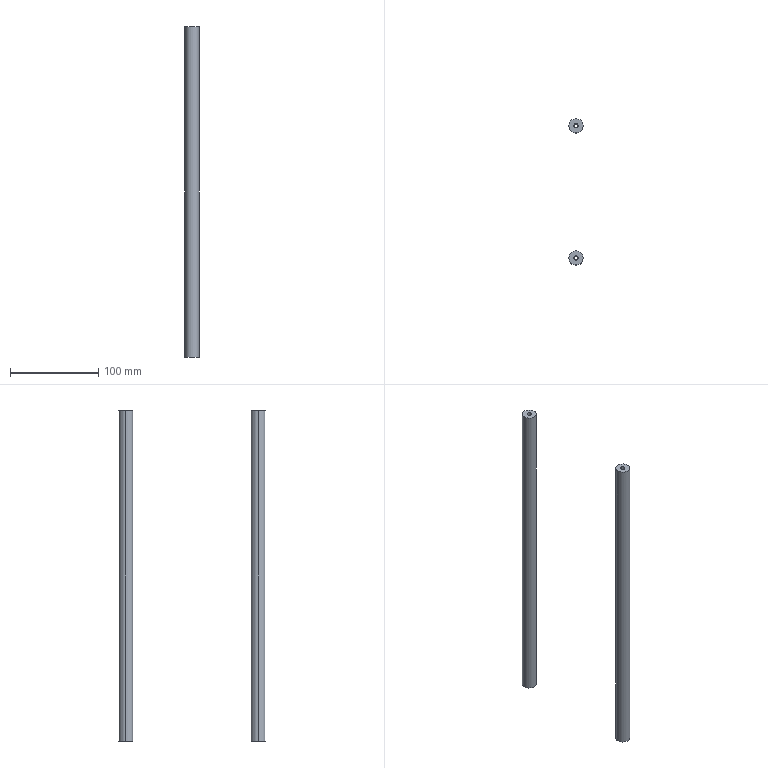Part | SolidWorks | features Extrusion 1, HoleWzd 1 | 2 solids | 12 faces | box 16 x 166 x 375 mm | volume 136070 mm3 | cylinder 8 | plane 4 | commonest cylinder face diameters 5 x4 16 x4
STEP:
#1=CARTESIAN_POINT('',(-75.5,75.,375.));
#2=VERTEX_POINT('',#1);
#3=CARTESIAN_POINT('',(-80.5,75.,375.));
#4=VERTEX_POINT('',#3);
#5=CARTESIAN_POINT('',(-78.,75.,375.));
#6=DIRECTION('',(0.,0.,-1.));
#7=DIRECTION('',(-1.,0.,0.));
#8=AXIS2_PLACEMENT_3D('',#5,#6,#7);
#9=CIRCLE('',#8,2.5);
#10=EDGE_CURVE('',#2,#4,#9,.T.);
#11=ORIENTED_EDGE('',*,*,#10,.F.);
#12=CARTESIAN_POINT('',(-75.5,75.,0.));
#13=VERTEX_POINT('',#12);
#14=CARTESIAN_POINT('',(-75.5,75.,0.));
#15=DIRECTION('',(0.,0.,-1.));
#16=VECTOR('',#15,1000.);
#17=LINE('',#14,#16);
#18=EDGE_CURVE('',#2,#13,#17,.T.);
#19=ORIENTED_EDGE('',*,*,#18,.T.);
#20=CARTESIAN_POINT('',(-80.5,75.,0.));
#21=VERTEX_POINT('',#20);
#22=CARTESIAN_POINT('',(-78.,75.,0.));
#23=DIRECTION('',(0.,0.,-1.));
#24=DIRECTION('',(-1.,0.,0.));
#25=AXIS2_PLACEMENT_3D('',#22,#23,#24);
#26=CIRCLE('',#25,2.5);
#27=EDGE_CURVE('',#13,#21,#26,.T.);
#28=ORIENTED_EDGE('',*,*,#27,.T.);
#29=CARTESIAN_POINT('',(-80.5,75.,0.));
#30=DIRECTION('',(0.,0.,-1.));
#31=VECTOR('',#30,1000.);
#32=LINE('',#29,#31);
#33=EDGE_CURVE('',#4,#21,#32,.T.);
#34=ORIENTED_EDGE('',*,*,#33,.F.);
#35=EDGE_LOOP('',(#11,#19,#28,#34));
#36=FACE_OUTER_BOUND('',#35,.T.);
#37=CARTESIAN_POINT('',(-78.,75.,0.));
#38=DIRECTION('',(0.,0.,-1.));
#39=DIRECTION('',(-1.,0.,0.));
#40=AXIS2_PLACEMENT_3D('',#37,#38,#39);
#41=CYLINDRICAL_SURFACE('',#40,2.5);
#42=ADVANCED_FACE('',(#36),#41,.F.);
#43=CARTESIAN_POINT('',(-70.,75.,375.));
#44=VERTEX_POINT('',#43);
#45=CARTESIAN_POINT('',(-86.,75.,375.));
#46=VERTEX_POINT('',#45);
#47=CARTESIAN_POINT('',(-78.,75.,375.));
#48=DIRECTION('',(0.,0.,1.));
#49=DIRECTION('',(1.,0.,0.));
#50=AXIS2_PLACEMENT_3D('',#47,#48,#49);
#51=CIRCLE('',#50,8.);
#52=EDGE_CURVE('',#44,#46,#51,.T.);
#53=ORIENTED_EDGE('',*,*,#52,.F.);
#54=CARTESIAN_POINT('',(-70.,75.,0.));
#55=VERTEX_POINT('',#54);
#56=CARTESIAN_POINT('',(-70.,75.,375.));
#57=DIRECTION('',(0.,0.,-1.));
#58=VECTOR('',#57,1000.);
#59=LINE('',#56,#58);
#60=EDGE_CURVE('',#44,#55,#59,.T.);
#61=ORIENTED_EDGE('',*,*,#60,.T.);
#62=CARTESIAN_POINT('',(-86.,75.,0.));
#63=VERTEX_POINT('',#62);
#64=CARTESIAN_POINT('',(-78.,75.,0.));
#65=DIRECTION('',(0.,0.,1.));
#66=DIRECTION('',(1.,0.,0.));
#67=AXIS2_PLACEMENT_3D('',#64,#65,#66);
#68=CIRCLE('',#67,8.);
#69=EDGE_CURVE('',#55,#63,#68,.T.);
#70=ORIENTED_EDGE('',*,*,#69,.T.);
#71=CARTESIAN_POINT('',(-86.,75.,375.));
#72=DIRECTION('',(0.,0.,-1.));
#73=VECTOR('',#72,1000.);
#74=LINE('',#71,#73);
#75=EDGE_CURVE('',#46,#63,#74,.T.);
#76=ORIENTED_EDGE('',*,*,#75,.F.);
#77=EDGE_LOOP('',(#53,#61,#70,#76));
#78=FACE_OUTER_BOUND('',#77,.T.);
#79=CARTESIAN_POINT('',(-78.,75.,375.));
#80=DIRECTION('',(0.,0.,-1.));
#81=DIRECTION('',(-1.,0.,0.));
#82=AXIS2_PLACEMENT_3D('',#79,#80,#81);
#83=CYLINDRICAL_SURFACE('',#82,8.);
#84=ADVANCED_FACE('',(#78),#83,.T.);
#85=ORIENTED_EDGE('',*,*,#60,.F.);
#86=CARTESIAN_POINT('',(-78.,75.,375.));
#87=DIRECTION('',(0.,0.,1.));
#88=DIRECTION('',(1.,0.,0.));
#89=AXIS2_PLACEMENT_3D('',#86,#87,#88);
#90=CIRCLE('',#89,8.);
#91=EDGE_CURVE('',#46,#44,#90,.T.);
#92=ORIENTED_EDGE('',*,*,#91,.F.);
#93=ORIENTED_EDGE('',*,*,#75,.T.);
#94=CARTESIAN_POINT('',(-78.,75.,0.));
#95=DIRECTION('',(0.,0.,1.));
#96=DIRECTION('',(1.,0.,0.));
#97=AXIS2_PLACEMENT_3D('',#94,#95,#96);
#98=CIRCLE('',#97,8.);
#99=EDGE_CURVE('',#63,#55,#98,.T.);
#100=ORIENTED_EDGE('',*,*,#99,.T.);
#101=EDGE_LOOP('',(#85,#92,#93,#100));
#102=FACE_OUTER_BOUND('',#101,.T.);
#103=CARTESIAN_POINT('',(-78.,75.,375.));
#104=DIRECTION('',(0.,0.,-1.));
#105=DIRECTION('',(-1.,0.,0.));
#106=AXIS2_PLACEMENT_3D('',#103,#104,#105);
#107=CYLINDRICAL_SURFACE('',#106,8.);
#108=ADVANCED_FACE('',(#102),#107,.T.);
#109=CARTESIAN_POINT('',(-78.,75.,375.));
#110=DIRECTION('',(0.,0.,-1.));
#111=DIRECTION('',(-1.,0.,0.));
#112=AXIS2_PLACEMENT_3D('',#109,#110,#111);
#113=CIRCLE('',#112,2.5);
#114=EDGE_CURVE('',#4,#2,#113,.T.);
#115=ORIENTED_EDGE('',*,*,#114,.T.);
#116=ORIENTED_EDGE('',*,*,#10,.T.);
#117=EDGE_LOOP('',(#115,#116));
#118=FACE_BOUND('',#117,.T.);
#119=ORIENTED_EDGE('',*,*,#91,.T.);
#120=ORIENTED_EDGE('',*,*,#52,.T.);
#121=EDGE_LOOP('',(#119,#120));
#122=FACE_OUTER_BOUND('',#121,.T.);
#123=CARTESIAN_POINT('',(-78.,75.,375.));
#124=DIRECTION('',(0.,0.,1.));
#125=DIRECTION('',(1.,0.,0.));
#126=AXIS2_PLACEMENT_3D('',#123,#124,#125);
#127=PLANE('',#126);
#128=ADVANCED_FACE('',(#118,#122),#127,.T.);
#129=CARTESIAN_POINT('',(-78.,75.,0.));
#130=DIRECTION('',(0.,0.,-1.));
#131=DIRECTION('',(-1.,0.,0.));
#132=AXIS2_PLACEMENT_3D('',#129,#130,#131);
#133=CIRCLE('',#132,2.5);
#134=EDGE_CURVE('',#21,#13,#133,.T.);
#135=ORIENTED_EDGE('',*,*,#134,.F.);
#136=ORIENTED_EDGE('',*,*,#27,.F.);
#137=EDGE_LOOP('',(#135,#136));
#138=FACE_BOUND('',#137,.T.);
#139=ORIENTED_EDGE('',*,*,#99,.F.);
#140=ORIENTED_EDGE('',*,*,#69,.F.);
#141=EDGE_LOOP('',(#139,#140));
#142=FACE_OUTER_BOUND('',#141,.T.);
#143=CARTESIAN_POINT('',(-78.,75.,0.));
#144=DIRECTION('',(0.,0.,1.));
#145=DIRECTION('',(1.,0.,0.));
#146=AXIS2_PLACEMENT_3D('',#143,#144,#145);
#147=PLANE('',#146);
#148=ADVANCED_FACE('',(#138,#142),#147,.F.);
#149=ORIENTED_EDGE('',*,*,#18,.F.);
#150=ORIENTED_EDGE('',*,*,#114,.F.);
#151=ORIENTED_EDGE('',*,*,#33,.T.);
#152=ORIENTED_EDGE('',*,*,#134,.T.);
#153=EDGE_LOOP('',(#149,#150,#151,#152));
#154=FACE_OUTER_BOUND('',#153,.T.);
#155=CARTESIAN_POINT('',(-78.,75.,0.));
#156=DIRECTION('',(0.,0.,-1.));
#157=DIRECTION('',(-1.,0.,0.));
#158=AXIS2_PLACEMENT_3D('',#155,#156,#157);
#159=CYLINDRICAL_SURFACE('',#158,2.5);
#160=ADVANCED_FACE('',(#154),#159,.F.);
#161=CLOSED_SHELL('',(#42,#84,#108,#128,#148,#160));
#162=MANIFOLD_SOLID_BREP('',#161);
#163=CARTESIAN_POINT('',(-75.5,-75.,375.));
#164=VERTEX_POINT('',#163);
#165=CARTESIAN_POINT('',(-80.5,-75.,375.));
#166=VERTEX_POINT('',#165);
#167=CARTESIAN_POINT('',(-78.,-75.,375.));
#168=DIRECTION('',(0.,0.,-1.));
#169=DIRECTION('',(-1.,0.,0.));
#170=AXIS2_PLACEMENT_3D('',#167,#168,#169);
#171=CIRCLE('',#170,2.5);
#172=EDGE_CURVE('',#164,#166,#171,.T.);
#173=ORIENTED_EDGE('',*,*,#172,.F.);
#174=CARTESIAN_POINT('',(-75.5,-75.,0.));
#175=VERTEX_POINT('',#174);
#176=CARTESIAN_POINT('',(-75.5,-75.,0.));
#177=DIRECTION('',(0.,0.,-1.));
#178=VECTOR('',#177,1000.);
#179=LINE('',#176,#178);
#180=EDGE_CURVE('',#164,#175,#179,.T.);
#181=ORIENTED_EDGE('',*,*,#180,.T.);
#182=CARTESIAN_POINT('',(-80.5,-75.,0.));
#183=VERTEX_POINT('',#182);
#184=CARTESIAN_POINT('',(-78.,-75.,0.));
#185=DIRECTION('',(0.,0.,-1.));
#186=DIRECTION('',(-1.,0.,0.));
#187=AXIS2_PLACEMENT_3D('',#184,#185,#186);
#188=CIRCLE('',#187,2.5);
#189=EDGE_CURVE('',#175,#183,#188,.T.);
#190=ORIENTED_EDGE('',*,*,#189,.T.);
#191=CARTESIAN_POINT('',(-80.5,-75.,0.));
#192=DIRECTION('',(0.,0.,-1.));
#193=VECTOR('',#192,1000.);
#194=LINE('',#191,#193);
#195=EDGE_CURVE('',#166,#183,#194,.T.);
#196=ORIENTED_EDGE('',*,*,#195,.F.);
#197=EDGE_LOOP('',(#173,#181,#190,#196));
#198=FACE_OUTER_BOUND('',#197,.T.);
#199=CARTESIAN_POINT('',(-78.,-75.,0.));
#200=DIRECTION('',(0.,0.,-1.));
#201=DIRECTION('',(-1.,0.,0.));
#202=AXIS2_PLACEMENT_3D('',#199,#200,#201);
#203=CYLINDRICAL_SURFACE('',#202,2.5);
#204=ADVANCED_FACE('',(#198),#203,.F.);
#205=CARTESIAN_POINT('',(-70.,-75.,375.));
#206=VERTEX_POINT('',#205);
#207=CARTESIAN_POINT('',(-86.,-75.,375.));
#208=VERTEX_POINT('',#207);
#209=CARTESIAN_POINT('',(-78.,-75.,375.));
#210=DIRECTION('',(0.,0.,1.));
#211=DIRECTION('',(-1.,0.,0.));
#212=AXIS2_PLACEMENT_3D('',#209,#210,#211);
#213=CIRCLE('',#212,8.);
#214=EDGE_CURVE('',#206,#208,#213,.T.);
#215=ORIENTED_EDGE('',*,*,#214,.F.);
#216=CARTESIAN_POINT('',(-70.,-75.,0.));
#217=VERTEX_POINT('',#216);
#218=CARTESIAN_POINT('',(-70.,-75.,375.));
#219=DIRECTION('',(0.,0.,-1.));
#220=VECTOR('',#219,1000.);
#221=LINE('',#218,#220);
#222=EDGE_CURVE('',#206,#217,#221,.T.);
#223=ORIENTED_EDGE('',*,*,#222,.T.);
#224=CARTESIAN_POINT('',(-86.,-75.,0.));
#225=VERTEX_POINT('',#224);
#226=CARTESIAN_POINT('',(-78.,-75.,0.));
#227=DIRECTION('',(0.,0.,1.));
#228=DIRECTION('',(-1.,0.,0.));
#229=AXIS2_PLACEMENT_3D('',#226,#227,#228);
#230=CIRCLE('',#229,8.);
#231=EDGE_CURVE('',#217,#225,#230,.T.);
#232=ORIENTED_EDGE('',*,*,#231,.T.);
#233=CARTESIAN_POINT('',(-86.,-75.,375.));
#234=DIRECTION('',(0.,0.,-1.));
#235=VECTOR('',#234,1000.);
#236=LINE('',#233,#235);
#237=EDGE_CURVE('',#208,#225,#236,.T.);
#238=ORIENTED_EDGE('',*,*,#237,.F.);
#239=EDGE_LOOP('',(#215,#223,#232,#238));
#240=FACE_OUTER_BOUND('',#239,.T.);
#241=CARTESIAN_POINT('',(-78.,-75.,375.));
#242=DIRECTION('',(0.,0.,-1.));
#243=DIRECTION('',(-1.,0.,0.));
#244=AXIS2_PLACEMENT_3D('',#241,#242,#243);
#245=CYLINDRICAL_SURFACE('',#244,8.);
#246=ADVANCED_FACE('',(#240),#245,.T.);
#247=ORIENTED_EDGE('',*,*,#222,.F.);
#248=CARTESIAN_POINT('',(-78.,-75.,375.));
#249=DIRECTION('',(0.,0.,1.));
#250=DIRECTION('',(-1.,0.,0.));
#251=AXIS2_PLACEMENT_3D('',#248,#249,#250);
#252=CIRCLE('',#251,8.);
#253=EDGE_CURVE('',#208,#206,#252,.T.);
#254=ORIENTED_EDGE('',*,*,#253,.F.);
#255=ORIENTED_EDGE('',*,*,#237,.T.);
#256=CARTESIAN_POINT('',(-78.,-75.,0.));
#257=DIRECTION('',(0.,0.,1.));
#258=DIRECTION('',(-1.,0.,0.));
#259=AXIS2_PLACEMENT_3D('',#256,#257,#258);
#260=CIRCLE('',#259,8.);
#261=EDGE_CURVE('',#225,#217,#260,.T.);
#262=ORIENTED_EDGE('',*,*,#261,.T.);
#263=EDGE_LOOP('',(#247,#254,#255,#262));
#264=FACE_OUTER_BOUND('',#263,.T.);
#265=CARTESIAN_POINT('',(-78.,-75.,375.));
#266=DIRECTION('',(0.,0.,-1.));
#267=DIRECTION('',(-1.,0.,0.));
#268=AXIS2_PLACEMENT_3D('',#265,#266,#267);
#269=CYLINDRICAL_SURFACE('',#268,8.);
#270=ADVANCED_FACE('',(#264),#269,.T.);
#271=CARTESIAN_POINT('',(-78.,-75.,375.));
#272=DIRECTION('',(0.,0.,-1.));
#273=DIRECTION('',(-1.,0.,0.));
#274=AXIS2_PLACEMENT_3D('',#271,#272,#273);
#275=CIRCLE('',#274,2.5);
#276=EDGE_CURVE('',#166,#164,#275,.T.);
#277=ORIENTED_EDGE('',*,*,#276,.T.);
#278=ORIENTED_EDGE('',*,*,#172,.T.);
#279=EDGE_LOOP('',(#277,#278));
#280=FACE_BOUND('',#279,.T.);
#281=ORIENTED_EDGE('',*,*,#253,.T.);
#282=ORIENTED_EDGE('',*,*,#214,.T.);
#283=EDGE_LOOP('',(#281,#282));
#284=FACE_OUTER_BOUND('',#283,.T.);
#285=CARTESIAN_POINT('',(-78.,-75.,375.));
#286=DIRECTION('',(0.,0.,-1.));
#287=DIRECTION('',(-1.,0.,0.));
#288=AXIS2_PLACEMENT_3D('',#285,#286,#287);
#289=PLANE('',#288);
#290=ADVANCED_FACE('',(#280,#284),#289,.F.);
#291=CARTESIAN_POINT('',(-78.,-75.,0.));
#292=DIRECTION('',(0.,0.,-1.));
#293=DIRECTION('',(-1.,0.,0.));
#294=AXIS2_PLACEMENT_3D('',#291,#292,#293);
#295=CIRCLE('',#294,2.5);
#296=EDGE_CURVE('',#183,#175,#295,.T.);
#297=ORIENTED_EDGE('',*,*,#296,.F.);
#298=ORIENTED_EDGE('',*,*,#189,.F.);
#299=EDGE_LOOP('',(#297,#298));
#300=FACE_BOUND('',#299,.T.);
#301=ORIENTED_EDGE('',*,*,#261,.F.);
#302=ORIENTED_EDGE('',*,*,#231,.F.);
#303=EDGE_LOOP('',(#301,#302));
#304=FACE_OUTER_BOUND('',#303,.T.);
#305=CARTESIAN_POINT('',(-78.,-75.,0.));
#306=DIRECTION('',(0.,0.,-1.));
#307=DIRECTION('',(-1.,0.,0.));
#308=AXIS2_PLACEMENT_3D('',#305,#306,#307);
#309=PLANE('',#308);
#310=ADVANCED_FACE('',(#300,#304),#309,.T.);
#311=ORIENTED_EDGE('',*,*,#180,.F.);
#312=ORIENTED_EDGE('',*,*,#276,.F.);
#313=ORIENTED_EDGE('',*,*,#195,.T.);
#314=ORIENTED_EDGE('',*,*,#296,.T.);
#315=EDGE_LOOP('',(#311,#312,#313,#314));
#316=FACE_OUTER_BOUND('',#315,.T.);
#317=CARTESIAN_POINT('',(-78.,-75.,0.));
#318=DIRECTION('',(0.,0.,-1.));
#319=DIRECTION('',(-1.,0.,0.));
#320=AXIS2_PLACEMENT_3D('',#317,#318,#319);
#321=CYLINDRICAL_SURFACE('',#320,2.5);
#322=ADVANCED_FACE('',(#316),#321,.F.);
#323=CLOSED_SHELL('',(#204,#246,#270,#290,#310,#322));
#324=MANIFOLD_SOLID_BREP('',#323);
#325=CARTESIAN_POINT('',(0.,0.,0.));
#326=DIRECTION('',(0.,0.,1.));
#327=DIRECTION('',(1.,0.,0.));
#328=AXIS2_PLACEMENT_3D('',#325,#326,#327);
#329=(LENGTH_UNIT()NAMED_UNIT(*)SI_UNIT(.MILLI.,.METRE.));
#330=UNCERTAINTY_MEASURE_WITH_UNIT(LENGTH_MEASURE(0.00001),#329,'','');
#331=(NAMED_UNIT(*)PLANE_ANGLE_UNIT()SI_UNIT($,.RADIAN.));
#332=(NAMED_UNIT(*)SI_UNIT($,.STERADIAN.)SOLID_ANGLE_UNIT());
#333=(GEOMETRIC_REPRESENTATION_CONTEXT(3)GLOBAL_UNCERTAINTY_ASSIGNED_CONTEXT((#330))GLOBAL_UNIT_ASSIGNED_CONTEXT((#329,#331,#332))REPRESENTATION_CONTEXT('',''));
#334=ADVANCED_BREP_SHAPE_REPRESENTATION('',(#162,#324,#328),#333);